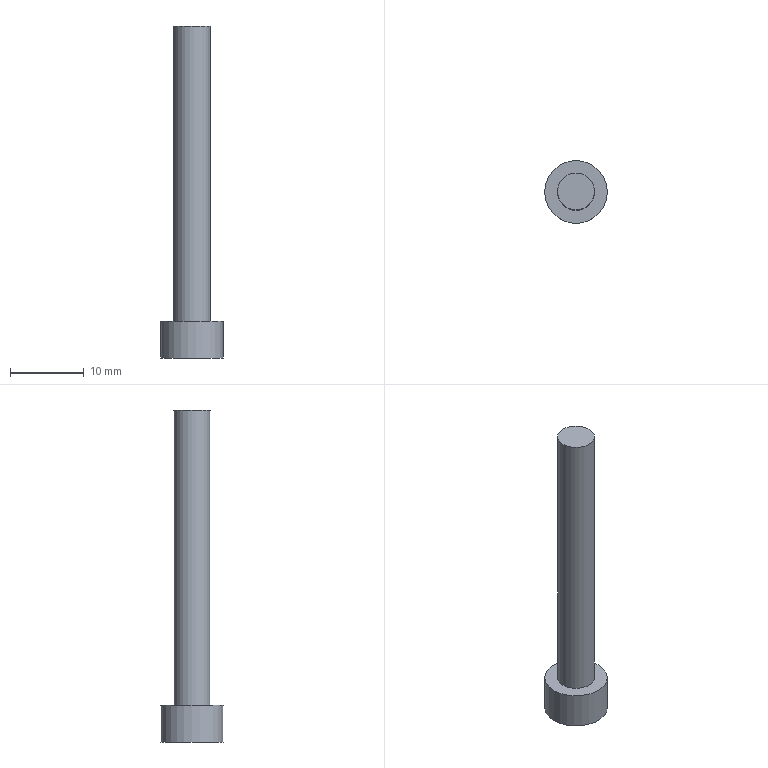Part | STEP file | 1 solid | 12 faces | box 8.5 x 8.5 x 45 mm | volume 1023 mm3 | plane 10 | cylinder 2 | commonest cylinder face diameters 5 x1 8.5 x1
STEP:
#1=CARTESIAN_POINT('',(0.,0.,0.));
#2=DIRECTION('',(0.,0.,1.));
#3=DIRECTION('',(1.,0.,0.));
#4=AXIS2_PLACEMENT_3D('',#1,#2,#3);
#5=CARTESIAN_POINT('',(1182.997,407.505,-56.381));
#6=VERTEX_POINT('',#5);
#7=CARTESIAN_POINT('',(1187.247,407.505,-56.381));
#8=DIRECTION('',(0.,0.,-1.));
#9=DIRECTION('',(-1.,0.,0.));
#10=AXIS2_PLACEMENT_3D('',#7,#8,#9);
#11=CIRCLE('',#10,4.25);
#12=CARTESIAN_POINT('',(1182.997,407.505,-56.381));
#13=DIRECTION('',(0.,0.,1.));
#14=DIRECTION('',(1.,0.,0.));
#15=AXIS2_PLACEMENT_3D('',#12,#13,#14);
#16=PLANE('',#15);
#17=CARTESIAN_POINT('',(0.,0.));
#18=CARTESIAN_POINT('',(0.,7.361));
#19=CARTESIAN_POINT('',(6.375,3.681));
#20=CARTESIAN_POINT('',(12.75,0.));
#21=CARTESIAN_POINT('',(6.375,-3.681));
#22=CARTESIAN_POINT('',(0.,-7.361));
#23=CARTESIAN_POINT('',(0.,0.));
#24=(BOUNDED_CURVE()B_SPLINE_CURVE(2,(#17,#18,#19,#20,#21,#22,#23),.UNSPECIFIED.,.T.,.F.)B_SPLINE_CURVE_WITH_KNOTS((1,2,2,2,2,1),(-2.094,0.,2.094,4.189,6.283,8.378),.UNSPECIFIED.)CURVE()GEOMETRIC_REPRESENTATION_ITEM()RATIONAL_B_SPLINE_CURVE((1.,0.5,1.,0.5,1.,0.5,1.))REPRESENTATION_ITEM(''));
#25=(GEOMETRIC_REPRESENTATION_CONTEXT(2)PARAMETRIC_REPRESENTATION_CONTEXT()REPRESENTATION_CONTEXT('',''));
#26=DEFINITIONAL_REPRESENTATION('',(#24),#25);
#27=PCURVE('',#16,#26);
#28=CARTESIAN_POINT('',(1187.247,407.505,-19.981));
#29=DIRECTION('',(0.,0.,-1.));
#30=DIRECTION('',(-1.,0.,0.));
#31=AXIS2_PLACEMENT_3D('',#28,#29,#30);
#32=CYLINDRICAL_SURFACE('',#31,4.25);
#33=CARTESIAN_POINT('',(0.,36.4));
#34=DIRECTION('',(1.,0.));
#35=VECTOR('',#34,1.);
#36=LINE('',#33,#35);
#37=(GEOMETRIC_REPRESENTATION_CONTEXT(2)PARAMETRIC_REPRESENTATION_CONTEXT()REPRESENTATION_CONTEXT('',''));
#38=DEFINITIONAL_REPRESENTATION('',(#36),#37);
#39=PCURVE('',#32,#38);
#40=SURFACE_CURVE('',#11,(#27,#39),.PCURVE_S1.);
#41=EDGE_CURVE('',#6,#6,#40,.T.);
#42=ORIENTED_EDGE('',*,*,#41,.T.);
#43=EDGE_LOOP('',(#42));
#44=FACE_BOUND('',#43,.T.);
#45=CARTESIAN_POINT('',(1188.402,409.505,-56.381));
#46=VERTEX_POINT('',#45);
#47=CARTESIAN_POINT('',(1186.092,409.505,-56.381));
#48=VERTEX_POINT('',#47);
#49=CARTESIAN_POINT('',(1188.402,409.505,-56.381));
#50=DIRECTION('',(-1.,0.,0.));
#51=VECTOR('',#50,1.);
#52=LINE('',#49,#51);
#53=CARTESIAN_POINT('',(5.405,2.));
#54=DIRECTION('',(-1.,0.));
#55=VECTOR('',#54,1.);
#56=LINE('',#53,#55);
#57=(GEOMETRIC_REPRESENTATION_CONTEXT(2)PARAMETRIC_REPRESENTATION_CONTEXT()REPRESENTATION_CONTEXT('',''));
#58=DEFINITIONAL_REPRESENTATION('',(#56),#57);
#59=PCURVE('',#16,#58);
#60=CARTESIAN_POINT('',(1188.402,409.505,-53.081));
#61=DIRECTION('',(0.,-1.,0.));
#62=DIRECTION('',(-1.,0.,0.));
#63=AXIS2_PLACEMENT_3D('',#60,#61,#62);
#64=PLANE('',#63);
#65=CARTESIAN_POINT('',(0.,3.3));
#66=DIRECTION('',(1.,0.));
#67=VECTOR('',#66,1.);
#68=LINE('',#65,#67);
#69=(GEOMETRIC_REPRESENTATION_CONTEXT(2)PARAMETRIC_REPRESENTATION_CONTEXT()REPRESENTATION_CONTEXT('',''));
#70=DEFINITIONAL_REPRESENTATION('',(#68),#69);
#71=PCURVE('',#64,#70);
#72=SURFACE_CURVE('',#52,(#59,#71),.PCURVE_S1.);
#73=EDGE_CURVE('',#46,#48,#72,.T.);
#74=ORIENTED_EDGE('',*,*,#73,.T.);
#75=CARTESIAN_POINT('',(1184.938,407.505,-56.381));
#76=VERTEX_POINT('',#75);
#77=CARTESIAN_POINT('',(1186.092,409.505,-56.381));
#78=DIRECTION('',(-0.5,-0.866,0.));
#79=VECTOR('',#78,1.);
#80=LINE('',#77,#79);
#81=CARTESIAN_POINT('',(3.095,2.));
#82=DIRECTION('',(-0.5,-0.866));
#83=VECTOR('',#82,1.);
#84=LINE('',#81,#83);
#85=(GEOMETRIC_REPRESENTATION_CONTEXT(2)PARAMETRIC_REPRESENTATION_CONTEXT()REPRESENTATION_CONTEXT('',''));
#86=DEFINITIONAL_REPRESENTATION('',(#84),#85);
#87=PCURVE('',#16,#86);
#88=CARTESIAN_POINT('',(1186.092,409.505,-53.081));
#89=DIRECTION('',(0.866,-0.5,0.));
#90=DIRECTION('',(-0.5,-0.866,0.));
#91=AXIS2_PLACEMENT_3D('',#88,#89,#90);
#92=PLANE('',#91);
#93=CARTESIAN_POINT('',(0.,3.3));
#94=DIRECTION('',(1.,0.));
#95=VECTOR('',#94,1.);
#96=LINE('',#93,#95);
#97=(GEOMETRIC_REPRESENTATION_CONTEXT(2)PARAMETRIC_REPRESENTATION_CONTEXT()REPRESENTATION_CONTEXT('',''));
#98=DEFINITIONAL_REPRESENTATION('',(#96),#97);
#99=PCURVE('',#92,#98);
#100=SURFACE_CURVE('',#80,(#87,#99),.PCURVE_S1.);
#101=EDGE_CURVE('',#48,#76,#100,.T.);
#102=ORIENTED_EDGE('',*,*,#101,.T.);
#103=CARTESIAN_POINT('',(1186.092,405.505,-56.381));
#104=VERTEX_POINT('',#103);
#105=CARTESIAN_POINT('',(1184.938,407.505,-56.381));
#106=DIRECTION('',(0.5,-0.866,0.));
#107=VECTOR('',#106,1.);
#108=LINE('',#105,#107);
#109=CARTESIAN_POINT('',(1.941,0.));
#110=DIRECTION('',(0.5,-0.866));
#111=VECTOR('',#110,1.);
#112=LINE('',#109,#111);
#113=(GEOMETRIC_REPRESENTATION_CONTEXT(2)PARAMETRIC_REPRESENTATION_CONTEXT()REPRESENTATION_CONTEXT('',''));
#114=DEFINITIONAL_REPRESENTATION('',(#112),#113);
#115=PCURVE('',#16,#114);
#116=CARTESIAN_POINT('',(1184.938,407.505,-53.081));
#117=DIRECTION('',(0.866,0.5,0.));
#118=DIRECTION('',(0.5,-0.866,0.));
#119=AXIS2_PLACEMENT_3D('',#116,#117,#118);
#120=PLANE('',#119);
#121=CARTESIAN_POINT('',(0.,3.3));
#122=DIRECTION('',(1.,0.));
#123=VECTOR('',#122,1.);
#124=LINE('',#121,#123);
#125=(GEOMETRIC_REPRESENTATION_CONTEXT(2)PARAMETRIC_REPRESENTATION_CONTEXT()REPRESENTATION_CONTEXT('',''));
#126=DEFINITIONAL_REPRESENTATION('',(#124),#125);
#127=PCURVE('',#120,#126);
#128=SURFACE_CURVE('',#108,(#115,#127),.PCURVE_S1.);
#129=EDGE_CURVE('',#76,#104,#128,.T.);
#130=ORIENTED_EDGE('',*,*,#129,.T.);
#131=CARTESIAN_POINT('',(1188.402,405.505,-56.381));
#132=VERTEX_POINT('',#131);
#133=CARTESIAN_POINT('',(1186.092,405.505,-56.381));
#134=DIRECTION('',(1.,0.,0.));
#135=VECTOR('',#134,1.);
#136=LINE('',#133,#135);
#137=CARTESIAN_POINT('',(3.095,-2.));
#138=DIRECTION('',(1.,0.));
#139=VECTOR('',#138,1.);
#140=LINE('',#137,#139);
#141=(GEOMETRIC_REPRESENTATION_CONTEXT(2)PARAMETRIC_REPRESENTATION_CONTEXT()REPRESENTATION_CONTEXT('',''));
#142=DEFINITIONAL_REPRESENTATION('',(#140),#141);
#143=PCURVE('',#16,#142);
#144=CARTESIAN_POINT('',(1186.092,405.505,-53.081));
#145=DIRECTION('',(0.,1.,0.));
#146=DIRECTION('',(0.,0.,-1.));
#147=AXIS2_PLACEMENT_3D('',#144,#145,#146);
#148=PLANE('',#147);
#149=CARTESIAN_POINT('',(3.3,0.));
#150=DIRECTION('',(0.,-1.));
#151=VECTOR('',#150,1.);
#152=LINE('',#149,#151);
#153=(GEOMETRIC_REPRESENTATION_CONTEXT(2)PARAMETRIC_REPRESENTATION_CONTEXT()REPRESENTATION_CONTEXT('',''));
#154=DEFINITIONAL_REPRESENTATION('',(#152),#153);
#155=PCURVE('',#148,#154);
#156=SURFACE_CURVE('',#136,(#143,#155),.PCURVE_S1.);
#157=EDGE_CURVE('',#104,#132,#156,.T.);
#158=ORIENTED_EDGE('',*,*,#157,.T.);
#159=CARTESIAN_POINT('',(1189.557,407.505,-56.381));
#160=VERTEX_POINT('',#159);
#161=CARTESIAN_POINT('',(1188.402,405.505,-56.381));
#162=DIRECTION('',(0.5,0.866,0.));
#163=VECTOR('',#162,1.);
#164=LINE('',#161,#163);
#165=CARTESIAN_POINT('',(5.405,-2.));
#166=DIRECTION('',(0.5,0.866));
#167=VECTOR('',#166,1.);
#168=LINE('',#165,#167);
#169=(GEOMETRIC_REPRESENTATION_CONTEXT(2)PARAMETRIC_REPRESENTATION_CONTEXT()REPRESENTATION_CONTEXT('',''));
#170=DEFINITIONAL_REPRESENTATION('',(#168),#169);
#171=PCURVE('',#16,#170);
#172=CARTESIAN_POINT('',(1188.402,405.505,-53.081));
#173=DIRECTION('',(-0.866,0.5,0.));
#174=DIRECTION('',(0.5,0.866,0.));
#175=AXIS2_PLACEMENT_3D('',#172,#173,#174);
#176=PLANE('',#175);
#177=CARTESIAN_POINT('',(0.,3.3));
#178=DIRECTION('',(1.,0.));
#179=VECTOR('',#178,1.);
#180=LINE('',#177,#179);
#181=(GEOMETRIC_REPRESENTATION_CONTEXT(2)PARAMETRIC_REPRESENTATION_CONTEXT()REPRESENTATION_CONTEXT('',''));
#182=DEFINITIONAL_REPRESENTATION('',(#180),#181);
#183=PCURVE('',#176,#182);
#184=SURFACE_CURVE('',#164,(#171,#183),.PCURVE_S1.);
#185=EDGE_CURVE('',#132,#160,#184,.T.);
#186=ORIENTED_EDGE('',*,*,#185,.T.);
#187=CARTESIAN_POINT('',(1189.557,407.505,-56.381));
#188=DIRECTION('',(-0.5,0.866,0.));
#189=VECTOR('',#188,1.);
#190=LINE('',#187,#189);
#191=CARTESIAN_POINT('',(6.559,0.));
#192=DIRECTION('',(-0.5,0.866));
#193=VECTOR('',#192,1.);
#194=LINE('',#191,#193);
#195=(GEOMETRIC_REPRESENTATION_CONTEXT(2)PARAMETRIC_REPRESENTATION_CONTEXT()REPRESENTATION_CONTEXT('',''));
#196=DEFINITIONAL_REPRESENTATION('',(#194),#195);
#197=PCURVE('',#16,#196);
#198=CARTESIAN_POINT('',(1189.557,407.505,-53.081));
#199=DIRECTION('',(-0.866,-0.5,0.));
#200=DIRECTION('',(-0.5,0.866,0.));
#201=AXIS2_PLACEMENT_3D('',#198,#199,#200);
#202=PLANE('',#201);
#203=CARTESIAN_POINT('',(0.,3.3));
#204=DIRECTION('',(1.,0.));
#205=VECTOR('',#204,1.);
#206=LINE('',#203,#205);
#207=(GEOMETRIC_REPRESENTATION_CONTEXT(2)PARAMETRIC_REPRESENTATION_CONTEXT()REPRESENTATION_CONTEXT('',''));
#208=DEFINITIONAL_REPRESENTATION('',(#206),#207);
#209=PCURVE('',#202,#208);
#210=SURFACE_CURVE('',#190,(#197,#209),.PCURVE_S1.);
#211=EDGE_CURVE('',#160,#46,#210,.T.);
#212=ORIENTED_EDGE('',*,*,#211,.T.);
#213=EDGE_LOOP('',(#74,#102,#130,#158,#186,#212));
#214=FACE_BOUND('',#213,.T.);
#215=ADVANCED_FACE('',(#44,#214),#16,.F.);
#216=ORIENTED_EDGE('',*,*,#41,.F.);
#217=CARTESIAN_POINT('',(1182.997,407.505,-51.381));
#218=VERTEX_POINT('',#217);
#219=CARTESIAN_POINT('',(1182.997,407.505,-51.381));
#220=CARTESIAN_POINT('',(1182.997,407.505,-56.381));
#221=B_SPLINE_CURVE_WITH_KNOTS('',1,(#219,#220),.UNSPECIFIED.,.F.,.F.,(2,2),(31.4,36.4),.PIECEWISE_BEZIER_KNOTS.);
#222=CARTESIAN_POINT('',(0.,0.));
#223=DIRECTION('',(0.,1.));
#224=VECTOR('',#223,1.);
#225=LINE('',#222,#224);
#226=(GEOMETRIC_REPRESENTATION_CONTEXT(2)PARAMETRIC_REPRESENTATION_CONTEXT()REPRESENTATION_CONTEXT('',''));
#227=DEFINITIONAL_REPRESENTATION('',(#225),#226);
#228=PCURVE('',#32,#227);
#229=CARTESIAN_POINT('',(6.283,0.));
#230=DIRECTION('',(0.,1.));
#231=VECTOR('',#230,1.);
#232=LINE('',#229,#231);
#233=(GEOMETRIC_REPRESENTATION_CONTEXT(2)PARAMETRIC_REPRESENTATION_CONTEXT()REPRESENTATION_CONTEXT('',''));
#234=DEFINITIONAL_REPRESENTATION('',(#232),#233);
#235=PCURVE('',#32,#234);
#236=SEAM_CURVE('',#221,(#228,#235),.PCURVE_S1.);
#237=EDGE_CURVE('',#218,#6,#236,.T.);
#238=ORIENTED_EDGE('',*,*,#237,.F.);
#239=CARTESIAN_POINT('',(1187.247,407.505,-51.381));
#240=DIRECTION('',(0.,0.,-1.));
#241=DIRECTION('',(-1.,0.,0.));
#242=AXIS2_PLACEMENT_3D('',#239,#240,#241);
#243=CIRCLE('',#242,4.25);
#244=CARTESIAN_POINT('',(0.,31.4));
#245=DIRECTION('',(1.,0.));
#246=VECTOR('',#245,1.);
#247=LINE('',#244,#246);
#248=(GEOMETRIC_REPRESENTATION_CONTEXT(2)PARAMETRIC_REPRESENTATION_CONTEXT()REPRESENTATION_CONTEXT('',''));
#249=DEFINITIONAL_REPRESENTATION('',(#247),#248);
#250=PCURVE('',#32,#249);
#251=CARTESIAN_POINT('',(1184.747,407.505,-51.381));
#252=DIRECTION('',(0.,0.,-1.));
#253=DIRECTION('',(-1.,0.,0.));
#254=AXIS2_PLACEMENT_3D('',#251,#252,#253);
#255=PLANE('',#254);
#256=CARTESIAN_POINT('',(-2.5,0.));
#257=DIRECTION('',(1.,0.));
#258=AXIS2_PLACEMENT_2D('',#256,#257);
#259=CIRCLE('',#258,4.25);
#260=(GEOMETRIC_REPRESENTATION_CONTEXT(2)PARAMETRIC_REPRESENTATION_CONTEXT()REPRESENTATION_CONTEXT('',''));
#261=DEFINITIONAL_REPRESENTATION('',(#259),#260);
#262=PCURVE('',#255,#261);
#263=SURFACE_CURVE('',#243,(#250,#262),.PCURVE_S1.);
#264=EDGE_CURVE('',#218,#218,#263,.T.);
#265=ORIENTED_EDGE('',*,*,#264,.T.);
#266=ORIENTED_EDGE('',*,*,#237,.T.);
#267=EDGE_LOOP('',(#216,#238,#265,#266));
#268=FACE_BOUND('',#267,.T.);
#269=ADVANCED_FACE('',(#268),#32,.T.);
#270=ORIENTED_EDGE('',*,*,#264,.F.);
#271=EDGE_LOOP('',(#270));
#272=FACE_BOUND('',#271,.T.);
#273=CARTESIAN_POINT('',(1184.747,407.505,-51.381));
#274=VERTEX_POINT('',#273);
#275=CARTESIAN_POINT('',(1187.247,407.505,-51.381));
#276=DIRECTION('',(0.,0.,-1.));
#277=DIRECTION('',(-1.,0.,0.));
#278=AXIS2_PLACEMENT_3D('',#275,#276,#277);
#279=CIRCLE('',#278,2.5);
#280=CARTESIAN_POINT('',(-2.5,0.));
#281=DIRECTION('',(1.,0.));
#282=AXIS2_PLACEMENT_2D('',#280,#281);
#283=CIRCLE('',#282,2.5);
#284=(GEOMETRIC_REPRESENTATION_CONTEXT(2)PARAMETRIC_REPRESENTATION_CONTEXT()REPRESENTATION_CONTEXT('',''));
#285=DEFINITIONAL_REPRESENTATION('',(#283),#284);
#286=PCURVE('',#255,#285);
#287=CARTESIAN_POINT('',(1187.247,407.505,-19.981));
#288=DIRECTION('',(0.,0.,-1.));
#289=DIRECTION('',(-1.,0.,0.));
#290=AXIS2_PLACEMENT_3D('',#287,#288,#289);
#291=CYLINDRICAL_SURFACE('',#290,2.5);
#292=CARTESIAN_POINT('',(0.,31.4));
#293=DIRECTION('',(1.,0.));
#294=VECTOR('',#293,1.);
#295=LINE('',#292,#294);
#296=(GEOMETRIC_REPRESENTATION_CONTEXT(2)PARAMETRIC_REPRESENTATION_CONTEXT()REPRESENTATION_CONTEXT('',''));
#297=DEFINITIONAL_REPRESENTATION('',(#295),#296);
#298=PCURVE('',#291,#297);
#299=SURFACE_CURVE('',#279,(#286,#298),.PCURVE_S1.);
#300=EDGE_CURVE('',#274,#274,#299,.T.);
#301=ORIENTED_EDGE('',*,*,#300,.T.);
#302=EDGE_LOOP('',(#301));
#303=FACE_BOUND('',#302,.T.);
#304=ADVANCED_FACE('',(#272,#303),#255,.F.);
#305=ORIENTED_EDGE('',*,*,#300,.F.);
#306=CARTESIAN_POINT('',(1184.747,407.505,-11.381));
#307=VERTEX_POINT('',#306);
#308=CARTESIAN_POINT('',(1184.747,407.505,-11.381));
#309=CARTESIAN_POINT('',(1184.747,407.505,-51.381));
#310=B_SPLINE_CURVE_WITH_KNOTS('',1,(#308,#309),.UNSPECIFIED.,.F.,.F.,(2,2),(-8.6,31.4),.PIECEWISE_BEZIER_KNOTS.);
#311=CARTESIAN_POINT('',(0.,0.));
#312=DIRECTION('',(0.,1.));
#313=VECTOR('',#312,1.);
#314=LINE('',#311,#313);
#315=(GEOMETRIC_REPRESENTATION_CONTEXT(2)PARAMETRIC_REPRESENTATION_CONTEXT()REPRESENTATION_CONTEXT('',''));
#316=DEFINITIONAL_REPRESENTATION('',(#314),#315);
#317=PCURVE('',#291,#316);
#318=CARTESIAN_POINT('',(6.283,0.));
#319=DIRECTION('',(0.,1.));
#320=VECTOR('',#319,1.);
#321=LINE('',#318,#320);
#322=(GEOMETRIC_REPRESENTATION_CONTEXT(2)PARAMETRIC_REPRESENTATION_CONTEXT()REPRESENTATION_CONTEXT('',''));
#323=DEFINITIONAL_REPRESENTATION('',(#321),#322);
#324=PCURVE('',#291,#323);
#325=SEAM_CURVE('',#310,(#317,#324),.PCURVE_S1.);
#326=EDGE_CURVE('',#307,#274,#325,.T.);
#327=ORIENTED_EDGE('',*,*,#326,.F.);
#328=CARTESIAN_POINT('',(1187.247,407.505,-11.381));
#329=DIRECTION('',(0.,0.,-1.));
#330=DIRECTION('',(-1.,0.,0.));
#331=AXIS2_PLACEMENT_3D('',#328,#329,#330);
#332=CIRCLE('',#331,2.5);
#333=CARTESIAN_POINT('',(0.,-8.6));
#334=DIRECTION('',(1.,0.));
#335=VECTOR('',#334,1.);
#336=LINE('',#333,#335);
#337=(GEOMETRIC_REPRESENTATION_CONTEXT(2)PARAMETRIC_REPRESENTATION_CONTEXT()REPRESENTATION_CONTEXT('',''));
#338=DEFINITIONAL_REPRESENTATION('',(#336),#337);
#339=PCURVE('',#291,#338);
#340=CARTESIAN_POINT('',(1187.247,407.505,-11.381));
#341=DIRECTION('',(0.,0.,-1.));
#342=DIRECTION('',(-1.,0.,0.));
#343=AXIS2_PLACEMENT_3D('',#340,#341,#342);
#344=PLANE('',#343);
#345=CARTESIAN_POINT('',(0.,0.));
#346=DIRECTION('',(1.,0.));
#347=AXIS2_PLACEMENT_2D('',#345,#346);
#348=CIRCLE('',#347,2.5);
#349=(GEOMETRIC_REPRESENTATION_CONTEXT(2)PARAMETRIC_REPRESENTATION_CONTEXT()REPRESENTATION_CONTEXT('',''));
#350=DEFINITIONAL_REPRESENTATION('',(#348),#349);
#351=PCURVE('',#344,#350);
#352=SURFACE_CURVE('',#332,(#339,#351),.PCURVE_S1.);
#353=EDGE_CURVE('',#307,#307,#352,.T.);
#354=ORIENTED_EDGE('',*,*,#353,.T.);
#355=ORIENTED_EDGE('',*,*,#326,.T.);
#356=EDGE_LOOP('',(#305,#327,#354,#355));
#357=FACE_BOUND('',#356,.T.);
#358=ADVANCED_FACE('',(#357),#291,.T.);
#359=ORIENTED_EDGE('',*,*,#353,.F.);
#360=EDGE_LOOP('',(#359));
#361=FACE_BOUND('',#360,.T.);
#362=ADVANCED_FACE('',(#361),#344,.F.);
#363=ORIENTED_EDGE('',*,*,#73,.F.);
#364=CARTESIAN_POINT('',(1188.402,409.505,-53.081));
#365=VERTEX_POINT('',#364);
#366=CARTESIAN_POINT('',(1188.402,409.505,-53.081));
#367=DIRECTION('',(0.,0.,1.));
#368=VECTOR('',#367,1.);
#369=LINE('',#366,#368);
#370=CARTESIAN_POINT('',(0.,0.));
#371=DIRECTION('',(0.,-1.));
#372=VECTOR('',#371,1.);
#373=LINE('',#370,#372);
#374=(GEOMETRIC_REPRESENTATION_CONTEXT(2)PARAMETRIC_REPRESENTATION_CONTEXT()REPRESENTATION_CONTEXT('',''));
#375=DEFINITIONAL_REPRESENTATION('',(#373),#374);
#376=PCURVE('',#64,#375);
#377=CARTESIAN_POINT('',(2.309,0.));
#378=DIRECTION('',(0.,-1.));
#379=VECTOR('',#378,1.);
#380=LINE('',#377,#379);
#381=(GEOMETRIC_REPRESENTATION_CONTEXT(2)PARAMETRIC_REPRESENTATION_CONTEXT()REPRESENTATION_CONTEXT('',''));
#382=DEFINITIONAL_REPRESENTATION('',(#380),#381);
#383=PCURVE('',#202,#382);
#384=SURFACE_CURVE('',#369,(#376,#383),.PCURVE_S1.);
#385=EDGE_CURVE('',#46,#365,#384,.T.);
#386=ORIENTED_EDGE('',*,*,#385,.T.);
#387=CARTESIAN_POINT('',(1186.092,409.505,-53.081));
#388=VERTEX_POINT('',#387);
#389=CARTESIAN_POINT('',(1188.402,409.505,-53.081));
#390=DIRECTION('',(1.,0.,0.));
#391=VECTOR('',#390,1.);
#392=LINE('',#389,#391);
#393=CARTESIAN_POINT('',(0.,0.));
#394=DIRECTION('',(-1.,0.));
#395=VECTOR('',#394,1.);
#396=LINE('',#393,#395);
#397=(GEOMETRIC_REPRESENTATION_CONTEXT(2)PARAMETRIC_REPRESENTATION_CONTEXT()REPRESENTATION_CONTEXT('',''));
#398=DEFINITIONAL_REPRESENTATION('',(#396),#397);
#399=PCURVE('',#64,#398);
#400=CARTESIAN_POINT('',(1187.247,407.505,-53.081));
#401=DIRECTION('',(0.,0.,1.));
#402=DIRECTION('',(1.,0.,0.));
#403=AXIS2_PLACEMENT_3D('',#400,#401,#402);
#404=PLANE('',#403);
#405=CARTESIAN_POINT('',(1.155,2.));
#406=DIRECTION('',(1.,0.));
#407=VECTOR('',#406,1.);
#408=LINE('',#405,#407);
#409=(GEOMETRIC_REPRESENTATION_CONTEXT(2)PARAMETRIC_REPRESENTATION_CONTEXT()REPRESENTATION_CONTEXT('',''));
#410=DEFINITIONAL_REPRESENTATION('',(#408),#409);
#411=PCURVE('',#404,#410);
#412=SURFACE_CURVE('',#392,(#399,#411),.PCURVE_S1.);
#413=EDGE_CURVE('',#388,#365,#412,.T.);
#414=ORIENTED_EDGE('',*,*,#413,.F.);
#415=CARTESIAN_POINT('',(1186.092,409.505,-53.081));
#416=DIRECTION('',(0.,0.,1.));
#417=VECTOR('',#416,1.);
#418=LINE('',#415,#417);
#419=CARTESIAN_POINT('',(2.309,0.));
#420=DIRECTION('',(0.,-1.));
#421=VECTOR('',#420,1.);
#422=LINE('',#419,#421);
#423=(GEOMETRIC_REPRESENTATION_CONTEXT(2)PARAMETRIC_REPRESENTATION_CONTEXT()REPRESENTATION_CONTEXT('',''));
#424=DEFINITIONAL_REPRESENTATION('',(#422),#423);
#425=PCURVE('',#64,#424);
#426=CARTESIAN_POINT('',(0.,0.));
#427=DIRECTION('',(0.,-1.));
#428=VECTOR('',#427,1.);
#429=LINE('',#426,#428);
#430=(GEOMETRIC_REPRESENTATION_CONTEXT(2)PARAMETRIC_REPRESENTATION_CONTEXT()REPRESENTATION_CONTEXT('',''));
#431=DEFINITIONAL_REPRESENTATION('',(#429),#430);
#432=PCURVE('',#92,#431);
#433=SURFACE_CURVE('',#418,(#425,#432),.PCURVE_S1.);
#434=EDGE_CURVE('',#48,#388,#433,.T.);
#435=ORIENTED_EDGE('',*,*,#434,.F.);
#436=EDGE_LOOP('',(#363,#386,#414,#435));
#437=FACE_BOUND('',#436,.T.);
#438=ADVANCED_FACE('',(#437),#64,.T.);
#439=ORIENTED_EDGE('',*,*,#101,.F.);
#440=ORIENTED_EDGE('',*,*,#434,.T.);
#441=CARTESIAN_POINT('',(1184.938,407.505,-53.081));
#442=VERTEX_POINT('',#441);
#443=CARTESIAN_POINT('',(1186.092,409.505,-53.081));
#444=DIRECTION('',(0.5,0.866,0.));
#445=VECTOR('',#444,1.);
#446=LINE('',#443,#445);
#447=CARTESIAN_POINT('',(0.,0.));
#448=DIRECTION('',(-1.,0.));
#449=VECTOR('',#448,1.);
#450=LINE('',#447,#449);
#451=(GEOMETRIC_REPRESENTATION_CONTEXT(2)PARAMETRIC_REPRESENTATION_CONTEXT()REPRESENTATION_CONTEXT('',''));
#452=DEFINITIONAL_REPRESENTATION('',(#450),#451);
#453=PCURVE('',#92,#452);
#454=CARTESIAN_POINT('',(-1.155,2.));
#455=DIRECTION('',(0.5,0.866));
#456=VECTOR('',#455,1.);
#457=LINE('',#454,#456);
#458=(GEOMETRIC_REPRESENTATION_CONTEXT(2)PARAMETRIC_REPRESENTATION_CONTEXT()REPRESENTATION_CONTEXT('',''));
#459=DEFINITIONAL_REPRESENTATION('',(#457),#458);
#460=PCURVE('',#404,#459);
#461=SURFACE_CURVE('',#446,(#453,#460),.PCURVE_S1.);
#462=EDGE_CURVE('',#442,#388,#461,.T.);
#463=ORIENTED_EDGE('',*,*,#462,.F.);
#464=CARTESIAN_POINT('',(1184.938,407.505,-53.081));
#465=DIRECTION('',(0.,0.,1.));
#466=VECTOR('',#465,1.);
#467=LINE('',#464,#466);
#468=CARTESIAN_POINT('',(2.309,0.));
#469=DIRECTION('',(0.,-1.));
#470=VECTOR('',#469,1.);
#471=LINE('',#468,#470);
#472=(GEOMETRIC_REPRESENTATION_CONTEXT(2)PARAMETRIC_REPRESENTATION_CONTEXT()REPRESENTATION_CONTEXT('',''));
#473=DEFINITIONAL_REPRESENTATION('',(#471),#472);
#474=PCURVE('',#92,#473);
#475=CARTESIAN_POINT('',(0.,0.));
#476=DIRECTION('',(0.,-1.));
#477=VECTOR('',#476,1.);
#478=LINE('',#475,#477);
#479=(GEOMETRIC_REPRESENTATION_CONTEXT(2)PARAMETRIC_REPRESENTATION_CONTEXT()REPRESENTATION_CONTEXT('',''));
#480=DEFINITIONAL_REPRESENTATION('',(#478),#479);
#481=PCURVE('',#120,#480);
#482=SURFACE_CURVE('',#467,(#474,#481),.PCURVE_S1.);
#483=EDGE_CURVE('',#76,#442,#482,.T.);
#484=ORIENTED_EDGE('',*,*,#483,.F.);
#485=EDGE_LOOP('',(#439,#440,#463,#484));
#486=FACE_BOUND('',#485,.T.);
#487=ADVANCED_FACE('',(#486),#92,.T.);
#488=ORIENTED_EDGE('',*,*,#129,.F.);
#489=ORIENTED_EDGE('',*,*,#483,.T.);
#490=CARTESIAN_POINT('',(1186.092,405.505,-53.081));
#491=VERTEX_POINT('',#490);
#492=CARTESIAN_POINT('',(1184.938,407.505,-53.081));
#493=DIRECTION('',(-0.5,0.866,0.));
#494=VECTOR('',#493,1.);
#495=LINE('',#492,#494);
#496=CARTESIAN_POINT('',(0.,0.));
#497=DIRECTION('',(-1.,0.));
#498=VECTOR('',#497,1.);
#499=LINE('',#496,#498);
#500=(GEOMETRIC_REPRESENTATION_CONTEXT(2)PARAMETRIC_REPRESENTATION_CONTEXT()REPRESENTATION_CONTEXT('',''));
#501=DEFINITIONAL_REPRESENTATION('',(#499),#500);
#502=PCURVE('',#120,#501);
#503=CARTESIAN_POINT('',(-2.309,0.));
#504=DIRECTION('',(-0.5,0.866));
#505=VECTOR('',#504,1.);
#506=LINE('',#503,#505);
#507=(GEOMETRIC_REPRESENTATION_CONTEXT(2)PARAMETRIC_REPRESENTATION_CONTEXT()REPRESENTATION_CONTEXT('',''));
#508=DEFINITIONAL_REPRESENTATION('',(#506),#507);
#509=PCURVE('',#404,#508);
#510=SURFACE_CURVE('',#495,(#502,#509),.PCURVE_S1.);
#511=EDGE_CURVE('',#491,#442,#510,.T.);
#512=ORIENTED_EDGE('',*,*,#511,.F.);
#513=CARTESIAN_POINT('',(1186.092,405.505,-53.081));
#514=DIRECTION('',(0.,0.,1.));
#515=VECTOR('',#514,1.);
#516=LINE('',#513,#515);
#517=CARTESIAN_POINT('',(2.309,0.));
#518=DIRECTION('',(0.,-1.));
#519=VECTOR('',#518,1.);
#520=LINE('',#517,#519);
#521=(GEOMETRIC_REPRESENTATION_CONTEXT(2)PARAMETRIC_REPRESENTATION_CONTEXT()REPRESENTATION_CONTEXT('',''));
#522=DEFINITIONAL_REPRESENTATION('',(#520),#521);
#523=PCURVE('',#120,#522);
#524=CARTESIAN_POINT('',(0.,0.));
#525=DIRECTION('',(-1.,0.));
#526=VECTOR('',#525,1.);
#527=LINE('',#524,#526);
#528=(GEOMETRIC_REPRESENTATION_CONTEXT(2)PARAMETRIC_REPRESENTATION_CONTEXT()REPRESENTATION_CONTEXT('',''));
#529=DEFINITIONAL_REPRESENTATION('',(#527),#528);
#530=PCURVE('',#148,#529);
#531=SURFACE_CURVE('',#516,(#523,#530),.PCURVE_S1.);
#532=EDGE_CURVE('',#104,#491,#531,.T.);
#533=ORIENTED_EDGE('',*,*,#532,.F.);
#534=EDGE_LOOP('',(#488,#489,#512,#533));
#535=FACE_BOUND('',#534,.T.);
#536=ADVANCED_FACE('',(#535),#120,.T.);
#537=ORIENTED_EDGE('',*,*,#157,.F.);
#538=ORIENTED_EDGE('',*,*,#532,.T.);
#539=CARTESIAN_POINT('',(1188.402,405.505,-53.081));
#540=VERTEX_POINT('',#539);
#541=CARTESIAN_POINT('',(1186.092,405.505,-53.081));
#542=DIRECTION('',(-1.,0.,0.));
#543=VECTOR('',#542,1.);
#544=LINE('',#541,#543);
#545=CARTESIAN_POINT('',(0.,0.));
#546=DIRECTION('',(0.,1.));
#547=VECTOR('',#546,1.);
#548=LINE('',#545,#547);
#549=(GEOMETRIC_REPRESENTATION_CONTEXT(2)PARAMETRIC_REPRESENTATION_CONTEXT()REPRESENTATION_CONTEXT('',''));
#550=DEFINITIONAL_REPRESENTATION('',(#548),#549);
#551=PCURVE('',#148,#550);
#552=CARTESIAN_POINT('',(-1.155,-2.));
#553=DIRECTION('',(-1.,0.));
#554=VECTOR('',#553,1.);
#555=LINE('',#552,#554);
#556=(GEOMETRIC_REPRESENTATION_CONTEXT(2)PARAMETRIC_REPRESENTATION_CONTEXT()REPRESENTATION_CONTEXT('',''));
#557=DEFINITIONAL_REPRESENTATION('',(#555),#556);
#558=PCURVE('',#404,#557);
#559=SURFACE_CURVE('',#544,(#551,#558),.PCURVE_S1.);
#560=EDGE_CURVE('',#540,#491,#559,.T.);
#561=ORIENTED_EDGE('',*,*,#560,.F.);
#562=CARTESIAN_POINT('',(1188.402,405.505,-53.081));
#563=DIRECTION('',(0.,0.,1.));
#564=VECTOR('',#563,1.);
#565=LINE('',#562,#564);
#566=CARTESIAN_POINT('',(0.,-2.309));
#567=DIRECTION('',(-1.,0.));
#568=VECTOR('',#567,1.);
#569=LINE('',#566,#568);
#570=(GEOMETRIC_REPRESENTATION_CONTEXT(2)PARAMETRIC_REPRESENTATION_CONTEXT()REPRESENTATION_CONTEXT('',''));
#571=DEFINITIONAL_REPRESENTATION('',(#569),#570);
#572=PCURVE('',#148,#571);
#573=CARTESIAN_POINT('',(0.,0.));
#574=DIRECTION('',(0.,-1.));
#575=VECTOR('',#574,1.);
#576=LINE('',#573,#575);
#577=(GEOMETRIC_REPRESENTATION_CONTEXT(2)PARAMETRIC_REPRESENTATION_CONTEXT()REPRESENTATION_CONTEXT('',''));
#578=DEFINITIONAL_REPRESENTATION('',(#576),#577);
#579=PCURVE('',#176,#578);
#580=SURFACE_CURVE('',#565,(#572,#579),.PCURVE_S1.);
#581=EDGE_CURVE('',#132,#540,#580,.T.);
#582=ORIENTED_EDGE('',*,*,#581,.F.);
#583=EDGE_LOOP('',(#537,#538,#561,#582));
#584=FACE_BOUND('',#583,.T.);
#585=ADVANCED_FACE('',(#584),#148,.T.);
#586=ORIENTED_EDGE('',*,*,#185,.F.);
#587=ORIENTED_EDGE('',*,*,#581,.T.);
#588=CARTESIAN_POINT('',(1189.557,407.505,-53.081));
#589=VERTEX_POINT('',#588);
#590=CARTESIAN_POINT('',(1188.402,405.505,-53.081));
#591=DIRECTION('',(-0.5,-0.866,0.));
#592=VECTOR('',#591,1.);
#593=LINE('',#590,#592);
#594=CARTESIAN_POINT('',(0.,0.));
#595=DIRECTION('',(-1.,0.));
#596=VECTOR('',#595,1.);
#597=LINE('',#594,#596);
#598=(GEOMETRIC_REPRESENTATION_CONTEXT(2)PARAMETRIC_REPRESENTATION_CONTEXT()REPRESENTATION_CONTEXT('',''));
#599=DEFINITIONAL_REPRESENTATION('',(#597),#598);
#600=PCURVE('',#176,#599);
#601=CARTESIAN_POINT('',(1.155,-2.));
#602=DIRECTION('',(-0.5,-0.866));
#603=VECTOR('',#602,1.);
#604=LINE('',#601,#603);
#605=(GEOMETRIC_REPRESENTATION_CONTEXT(2)PARAMETRIC_REPRESENTATION_CONTEXT()REPRESENTATION_CONTEXT('',''));
#606=DEFINITIONAL_REPRESENTATION('',(#604),#605);
#607=PCURVE('',#404,#606);
#608=SURFACE_CURVE('',#593,(#600,#607),.PCURVE_S1.);
#609=EDGE_CURVE('',#589,#540,#608,.T.);
#610=ORIENTED_EDGE('',*,*,#609,.F.);
#611=CARTESIAN_POINT('',(1189.557,407.505,-53.081));
#612=DIRECTION('',(0.,0.,1.));
#613=VECTOR('',#612,1.);
#614=LINE('',#611,#613);
#615=CARTESIAN_POINT('',(2.309,0.));
#616=DIRECTION('',(0.,-1.));
#617=VECTOR('',#616,1.);
#618=LINE('',#615,#617);
#619=(GEOMETRIC_REPRESENTATION_CONTEXT(2)PARAMETRIC_REPRESENTATION_CONTEXT()REPRESENTATION_CONTEXT('',''));
#620=DEFINITIONAL_REPRESENTATION('',(#618),#619);
#621=PCURVE('',#176,#620);
#622=CARTESIAN_POINT('',(0.,0.));
#623=DIRECTION('',(0.,-1.));
#624=VECTOR('',#623,1.);
#625=LINE('',#622,#624);
#626=(GEOMETRIC_REPRESENTATION_CONTEXT(2)PARAMETRIC_REPRESENTATION_CONTEXT()REPRESENTATION_CONTEXT('',''));
#627=DEFINITIONAL_REPRESENTATION('',(#625),#626);
#628=PCURVE('',#202,#627);
#629=SURFACE_CURVE('',#614,(#621,#628),.PCURVE_S1.);
#630=EDGE_CURVE('',#160,#589,#629,.T.);
#631=ORIENTED_EDGE('',*,*,#630,.F.);
#632=EDGE_LOOP('',(#586,#587,#610,#631));
#633=FACE_BOUND('',#632,.T.);
#634=ADVANCED_FACE('',(#633),#176,.T.);
#635=ORIENTED_EDGE('',*,*,#211,.F.);
#636=ORIENTED_EDGE('',*,*,#630,.T.);
#637=CARTESIAN_POINT('',(1189.557,407.505,-53.081));
#638=DIRECTION('',(0.5,-0.866,0.));
#639=VECTOR('',#638,1.);
#640=LINE('',#637,#639);
#641=CARTESIAN_POINT('',(0.,0.));
#642=DIRECTION('',(-1.,0.));
#643=VECTOR('',#642,1.);
#644=LINE('',#641,#643);
#645=(GEOMETRIC_REPRESENTATION_CONTEXT(2)PARAMETRIC_REPRESENTATION_CONTEXT()REPRESENTATION_CONTEXT('',''));
#646=DEFINITIONAL_REPRESENTATION('',(#644),#645);
#647=PCURVE('',#202,#646);
#648=CARTESIAN_POINT('',(2.309,0.));
#649=DIRECTION('',(0.5,-0.866));
#650=VECTOR('',#649,1.);
#651=LINE('',#648,#650);
#652=(GEOMETRIC_REPRESENTATION_CONTEXT(2)PARAMETRIC_REPRESENTATION_CONTEXT()REPRESENTATION_CONTEXT('',''));
#653=DEFINITIONAL_REPRESENTATION('',(#651),#652);
#654=PCURVE('',#404,#653);
#655=SURFACE_CURVE('',#640,(#647,#654),.PCURVE_S1.);
#656=EDGE_CURVE('',#365,#589,#655,.T.);
#657=ORIENTED_EDGE('',*,*,#656,.F.);
#658=ORIENTED_EDGE('',*,*,#385,.F.);
#659=EDGE_LOOP('',(#635,#636,#657,#658));
#660=FACE_BOUND('',#659,.T.);
#661=ADVANCED_FACE('',(#660),#202,.T.);
#662=ORIENTED_EDGE('',*,*,#413,.T.);
#663=ORIENTED_EDGE('',*,*,#656,.T.);
#664=ORIENTED_EDGE('',*,*,#609,.T.);
#665=ORIENTED_EDGE('',*,*,#560,.T.);
#666=ORIENTED_EDGE('',*,*,#511,.T.);
#667=ORIENTED_EDGE('',*,*,#462,.T.);
#668=EDGE_LOOP('',(#662,#663,#664,#665,#666,#667));
#669=FACE_BOUND('',#668,.T.);
#670=ADVANCED_FACE('',(#669),#404,.F.);
#671=CLOSED_SHELL('',(#215,#269,#304,#358,#362,#438,#487,#536,#585,#634,#661,#670));
#672=MANIFOLD_SOLID_BREP('',#671);
#673=(LENGTH_UNIT()NAMED_UNIT(*)SI_UNIT(.MILLI.,.METRE.));
#674=UNCERTAINTY_MEASURE_WITH_UNIT(LENGTH_MEASURE(0.000002),#673,'','');
#675=(NAMED_UNIT(*)PLANE_ANGLE_UNIT()SI_UNIT($,.RADIAN.));
#676=(NAMED_UNIT(*)SI_UNIT($,.STERADIAN.)SOLID_ANGLE_UNIT());
#677=(GEOMETRIC_REPRESENTATION_CONTEXT(3)GLOBAL_UNCERTAINTY_ASSIGNED_CONTEXT((#674))GLOBAL_UNIT_ASSIGNED_CONTEXT((#673,#675,#676))REPRESENTATION_CONTEXT('',''));
#678=ADVANCED_BREP_SHAPE_REPRESENTATION('',(#4,#672),#677);